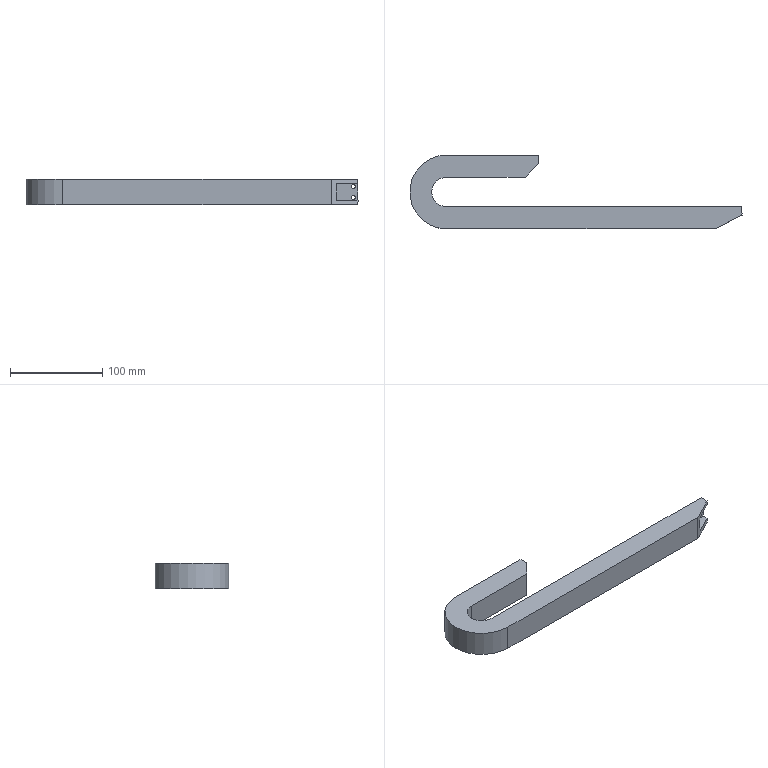Part | NX | 1 solid | 24 faces | box 360 x 80 x 28 mm | volume 171154 mm3 | plane 16 | cylinder 8 | commonest cylinder face diameters 4.5 x4 32 x1 38 x1 74 x1 80 x1
STEP:
#1=CARTESIAN_POINT('',(-232.,47.,-9.));
#2=VERTEX_POINT('',#1);
#3=CARTESIAN_POINT('',(-232.,47.,9.));
#4=VERTEX_POINT('',#3);
#5=CARTESIAN_POINT('',(-232.,47.,9.));
#6=DIRECTION('',(0.,0.,1.));
#7=VECTOR('',#6,1000.);
#8=LINE('',#5,#7);
#9=EDGE_CURVE('',#2,#4,#8,.T.);
#10=ORIENTED_EDGE('',*,*,#9,.F.);
#11=CARTESIAN_POINT('',(-320.,47.,-9.));
#12=VERTEX_POINT('',#11);
#13=CARTESIAN_POINT('',(-320.,47.,-9.));
#14=DIRECTION('',(1.,0.,0.));
#15=VECTOR('',#14,1000.);
#16=LINE('',#13,#15);
#17=EDGE_CURVE('',#12,#2,#16,.T.);
#18=ORIENTED_EDGE('',*,*,#17,.F.);
#19=CARTESIAN_POINT('',(-320.,47.,9.));
#20=VERTEX_POINT('',#19);
#21=CARTESIAN_POINT('',(-320.,47.,9.));
#22=DIRECTION('',(0.,0.,1.));
#23=VECTOR('',#22,1000.);
#24=LINE('',#21,#23);
#25=EDGE_CURVE('',#12,#20,#24,.T.);
#26=ORIENTED_EDGE('',*,*,#25,.T.);
#27=CARTESIAN_POINT('',(-320.,47.,9.));
#28=DIRECTION('',(1.,0.,0.));
#29=VECTOR('',#28,1000.);
#30=LINE('',#27,#29);
#31=EDGE_CURVE('',#20,#4,#30,.T.);
#32=ORIENTED_EDGE('',*,*,#31,.T.);
#33=EDGE_LOOP('',(#10,#18,#26,#32));
#34=FACE_BOUND('',#33,.T.);
#35=CARTESIAN_POINT('',(-320.,47.,9.));
#36=DIRECTION('',(0.,1.,0.));
#37=DIRECTION('',(0.,0.,1.));
#38=AXIS2_PLACEMENT_3D('',#35,#36,#37);
#39=PLANE('',#38);
#40=ADVANCED_FACE('',(#34),#39,.T.);
#41=CARTESIAN_POINT('',(-225.,65.,3.75));
#42=VERTEX_POINT('',#41);
#43=CARTESIAN_POINT('',(-225.,65.,6.));
#44=DIRECTION('',(0.,-1.,0.));
#45=DIRECTION('',(0.,0.,-1.));
#46=AXIS2_PLACEMENT_3D('',#43,#44,#45);
#47=CIRCLE('',#46,2.25);
#48=EDGE_CURVE('',#42,#42,#47,.T.);
#49=ORIENTED_EDGE('',*,*,#48,.F.);
#50=EDGE_LOOP('',(#49));
#51=FACE_BOUND('',#50,.T.);
#52=CARTESIAN_POINT('',(-225.,65.,-8.25));
#53=VERTEX_POINT('',#52);
#54=CARTESIAN_POINT('',(-225.,65.,-6.));
#55=DIRECTION('',(0.,-1.,0.));
#56=DIRECTION('',(0.,0.,-1.));
#57=AXIS2_PLACEMENT_3D('',#54,#55,#56);
#58=CIRCLE('',#57,2.25);
#59=EDGE_CURVE('',#53,#53,#58,.T.);
#60=ORIENTED_EDGE('',*,*,#59,.F.);
#61=EDGE_LOOP('',(#60));
#62=FACE_BOUND('',#61,.T.);
#63=CARTESIAN_POINT('',(-320.,65.,9.));
#64=VERTEX_POINT('',#63);
#65=CARTESIAN_POINT('',(-320.,65.,-9.));
#66=VERTEX_POINT('',#65);
#67=CARTESIAN_POINT('',(-320.,65.,9.));
#68=DIRECTION('',(0.,0.,-1.));
#69=VECTOR('',#68,1000.);
#70=LINE('',#67,#69);
#71=EDGE_CURVE('',#64,#66,#70,.T.);
#72=ORIENTED_EDGE('',*,*,#71,.T.);
#73=CARTESIAN_POINT('',(-220.,65.,-9.));
#74=VERTEX_POINT('',#73);
#75=CARTESIAN_POINT('',(-320.,65.,-9.));
#76=DIRECTION('',(1.,0.,0.));
#77=VECTOR('',#76,1000.);
#78=LINE('',#75,#77);
#79=EDGE_CURVE('',#66,#74,#78,.T.);
#80=ORIENTED_EDGE('',*,*,#79,.T.);
#81=CARTESIAN_POINT('',(-220.,65.,9.));
#82=VERTEX_POINT('',#81);
#83=CARTESIAN_POINT('',(-220.,65.,9.));
#84=DIRECTION('',(0.,0.,-1.));
#85=VECTOR('',#84,1000.);
#86=LINE('',#83,#85);
#87=EDGE_CURVE('',#82,#74,#86,.T.);
#88=ORIENTED_EDGE('',*,*,#87,.F.);
#89=CARTESIAN_POINT('',(-320.,65.,9.));
#90=DIRECTION('',(1.,0.,0.));
#91=VECTOR('',#90,1000.);
#92=LINE('',#89,#91);
#93=EDGE_CURVE('',#64,#82,#92,.T.);
#94=ORIENTED_EDGE('',*,*,#93,.F.);
#95=EDGE_LOOP('',(#72,#80,#88,#94));
#96=FACE_BOUND('',#95,.T.);
#97=CARTESIAN_POINT('',(-320.,65.,9.));
#98=DIRECTION('',(0.,-1.,0.));
#99=DIRECTION('',(0.,0.,-1.));
#100=AXIS2_PLACEMENT_3D('',#97,#98,#99);
#101=PLANE('',#100);
#102=ADVANCED_FACE('',(#51,#62,#96),#101,.T.);
#103=CARTESIAN_POINT('',(-225.,68.,3.75));
#104=VERTEX_POINT('',#103);
#105=CARTESIAN_POINT('',(-225.,68.,6.));
#106=DIRECTION('',(0.,-1.,0.));
#107=DIRECTION('',(0.,0.,-1.));
#108=AXIS2_PLACEMENT_3D('',#105,#106,#107);
#109=CIRCLE('',#108,2.25);
#110=EDGE_CURVE('',#104,#104,#109,.T.);
#111=ORIENTED_EDGE('',*,*,#110,.T.);
#112=EDGE_LOOP('',(#111));
#113=FACE_BOUND('',#112,.T.);
#114=CARTESIAN_POINT('',(-225.,68.,-8.25));
#115=VERTEX_POINT('',#114);
#116=CARTESIAN_POINT('',(-225.,68.,-6.));
#117=DIRECTION('',(0.,-1.,0.));
#118=DIRECTION('',(0.,0.,-1.));
#119=AXIS2_PLACEMENT_3D('',#116,#117,#118);
#120=CIRCLE('',#119,2.25);
#121=EDGE_CURVE('',#115,#115,#120,.T.);
#122=ORIENTED_EDGE('',*,*,#121,.T.);
#123=EDGE_LOOP('',(#122));
#124=FACE_BOUND('',#123,.T.);
#125=CARTESIAN_POINT('',(-320.,68.,14.));
#126=VERTEX_POINT('',#125);
#127=CARTESIAN_POINT('',(-320.,68.,-14.));
#128=VERTEX_POINT('',#127);
#129=CARTESIAN_POINT('',(-320.,68.,14.));
#130=DIRECTION('',(0.,0.,-1.));
#131=VECTOR('',#130,1000.);
#132=LINE('',#129,#131);
#133=EDGE_CURVE('',#126,#128,#132,.T.);
#134=ORIENTED_EDGE('',*,*,#133,.F.);
#135=CARTESIAN_POINT('',(-220.,68.,14.));
#136=VERTEX_POINT('',#135);
#137=CARTESIAN_POINT('',(-320.,68.,14.));
#138=DIRECTION('',(1.,0.,0.));
#139=VECTOR('',#138,1000.);
#140=LINE('',#137,#139);
#141=EDGE_CURVE('',#126,#136,#140,.T.);
#142=ORIENTED_EDGE('',*,*,#141,.T.);
#143=CARTESIAN_POINT('',(-220.,68.,-14.));
#144=VERTEX_POINT('',#143);
#145=CARTESIAN_POINT('',(-220.,68.,14.));
#146=DIRECTION('',(0.,0.,-1.));
#147=VECTOR('',#146,1000.);
#148=LINE('',#145,#147);
#149=EDGE_CURVE('',#136,#144,#148,.T.);
#150=ORIENTED_EDGE('',*,*,#149,.T.);
#151=CARTESIAN_POINT('',(-320.,68.,-14.));
#152=DIRECTION('',(1.,0.,0.));
#153=VECTOR('',#152,1000.);
#154=LINE('',#151,#153);
#155=EDGE_CURVE('',#128,#144,#154,.T.);
#156=ORIENTED_EDGE('',*,*,#155,.F.);
#157=EDGE_LOOP('',(#134,#142,#150,#156));
#158=FACE_BOUND('',#157,.T.);
#159=CARTESIAN_POINT('',(-320.,68.,14.));
#160=DIRECTION('',(0.,-1.,0.));
#161=DIRECTION('',(0.,0.,-1.));
#162=AXIS2_PLACEMENT_3D('',#159,#160,#161);
#163=PLANE('',#162);
#164=ADVANCED_FACE('',(#113,#124,#158),#163,.F.);
#165=CARTESIAN_POINT('',(-320.,44.,-14.));
#166=VERTEX_POINT('',#165);
#167=CARTESIAN_POINT('',(-235.,44.,-14.));
#168=VERTEX_POINT('',#167);
#169=CARTESIAN_POINT('',(-320.,44.,-14.));
#170=DIRECTION('',(1.,0.,0.));
#171=VECTOR('',#170,1000.);
#172=LINE('',#169,#171);
#173=EDGE_CURVE('',#166,#168,#172,.T.);
#174=ORIENTED_EDGE('',*,*,#173,.T.);
#175=CARTESIAN_POINT('',(-235.,44.,14.));
#176=VERTEX_POINT('',#175);
#177=CARTESIAN_POINT('',(-235.,44.,14.));
#178=DIRECTION('',(0.,0.,-1.));
#179=VECTOR('',#178,1000.);
#180=LINE('',#177,#179);
#181=EDGE_CURVE('',#176,#168,#180,.T.);
#182=ORIENTED_EDGE('',*,*,#181,.F.);
#183=CARTESIAN_POINT('',(-320.,44.,14.));
#184=VERTEX_POINT('',#183);
#185=CARTESIAN_POINT('',(-320.,44.,14.));
#186=DIRECTION('',(1.,0.,0.));
#187=VECTOR('',#186,1000.);
#188=LINE('',#185,#187);
#189=EDGE_CURVE('',#184,#176,#188,.T.);
#190=ORIENTED_EDGE('',*,*,#189,.F.);
#191=CARTESIAN_POINT('',(-320.,44.,14.));
#192=DIRECTION('',(0.,0.,1.));
#193=VECTOR('',#192,1000.);
#194=LINE('',#191,#193);
#195=EDGE_CURVE('',#166,#184,#194,.T.);
#196=ORIENTED_EDGE('',*,*,#195,.F.);
#197=EDGE_LOOP('',(#174,#182,#190,#196));
#198=FACE_BOUND('',#197,.T.);
#199=CARTESIAN_POINT('',(-320.,44.,14.));
#200=DIRECTION('',(0.,1.,0.));
#201=DIRECTION('',(0.,0.,1.));
#202=AXIS2_PLACEMENT_3D('',#199,#200,#201);
#203=PLANE('',#202);
#204=ADVANCED_FACE('',(#198),#203,.F.);
#205=CARTESIAN_POINT('',(-320.,9.,-9.));
#206=VERTEX_POINT('',#205);
#207=CARTESIAN_POINT('',(-320.,9.,9.));
#208=VERTEX_POINT('',#207);
#209=CARTESIAN_POINT('',(-320.,9.,9.));
#210=DIRECTION('',(0.,0.,1.));
#211=VECTOR('',#210,1000.);
#212=LINE('',#209,#211);
#213=EDGE_CURVE('',#206,#208,#212,.T.);
#214=ORIENTED_EDGE('',*,*,#213,.T.);
#215=CARTESIAN_POINT('',(-320.,28.,9.));
#216=DIRECTION('',(0.,0.,-1.));
#217=DIRECTION('',(-1.,0.,0.));
#218=AXIS2_PLACEMENT_3D('',#215,#216,#217);
#219=CIRCLE('',#218,19.);
#220=EDGE_CURVE('',#208,#20,#219,.T.);
#221=ORIENTED_EDGE('',*,*,#220,.T.);
#222=ORIENTED_EDGE('',*,*,#25,.F.);
#223=CARTESIAN_POINT('',(-320.,28.,-9.));
#224=DIRECTION('',(0.,0.,-1.));
#225=DIRECTION('',(-1.,0.,0.));
#226=AXIS2_PLACEMENT_3D('',#223,#224,#225);
#227=CIRCLE('',#226,19.);
#228=EDGE_CURVE('',#206,#12,#227,.T.);
#229=ORIENTED_EDGE('',*,*,#228,.F.);
#230=EDGE_LOOP('',(#214,#221,#222,#229));
#231=FACE_BOUND('',#230,.T.);
#232=CARTESIAN_POINT('',(-320.,28.,0.));
#233=DIRECTION('',(0.,0.,-1.));
#234=DIRECTION('',(-1.,0.,0.));
#235=AXIS2_PLACEMENT_3D('',#232,#233,#234);
#236=CYLINDRICAL_SURFACE('',#235,19.);
#237=ADVANCED_FACE('',(#231),#236,.T.);
#238=CARTESIAN_POINT('',(-320.,-9.,9.));
#239=VERTEX_POINT('',#238);
#240=CARTESIAN_POINT('',(-320.,-9.,-9.));
#241=VERTEX_POINT('',#240);
#242=CARTESIAN_POINT('',(-320.,-9.,9.));
#243=DIRECTION('',(0.,0.,-1.));
#244=VECTOR('',#243,1000.);
#245=LINE('',#242,#244);
#246=EDGE_CURVE('',#239,#241,#245,.T.);
#247=ORIENTED_EDGE('',*,*,#246,.T.);
#248=CARTESIAN_POINT('',(-320.,28.,-9.));
#249=DIRECTION('',(0.,0.,-1.));
#250=DIRECTION('',(-1.,0.,0.));
#251=AXIS2_PLACEMENT_3D('',#248,#249,#250);
#252=CIRCLE('',#251,37.);
#253=EDGE_CURVE('',#241,#66,#252,.T.);
#254=ORIENTED_EDGE('',*,*,#253,.T.);
#255=ORIENTED_EDGE('',*,*,#71,.F.);
#256=CARTESIAN_POINT('',(-320.,28.,9.));
#257=DIRECTION('',(0.,0.,-1.));
#258=DIRECTION('',(-1.,0.,0.));
#259=AXIS2_PLACEMENT_3D('',#256,#257,#258);
#260=CIRCLE('',#259,37.);
#261=EDGE_CURVE('',#239,#64,#260,.T.);
#262=ORIENTED_EDGE('',*,*,#261,.F.);
#263=EDGE_LOOP('',(#247,#254,#255,#262));
#264=FACE_BOUND('',#263,.T.);
#265=CARTESIAN_POINT('',(-320.,28.,0.));
#266=DIRECTION('',(0.,0.,-1.));
#267=DIRECTION('',(-1.,0.,0.));
#268=AXIS2_PLACEMENT_3D('',#265,#266,#267);
#269=CYLINDRICAL_SURFACE('',#268,37.);
#270=ADVANCED_FACE('',(#264),#269,.F.);
#271=CARTESIAN_POINT('',(-320.,-12.,14.));
#272=VERTEX_POINT('',#271);
#273=CARTESIAN_POINT('',(-320.,-12.,-14.));
#274=VERTEX_POINT('',#273);
#275=CARTESIAN_POINT('',(-320.,-12.,14.));
#276=DIRECTION('',(0.,0.,-1.));
#277=VECTOR('',#276,1000.);
#278=LINE('',#275,#277);
#279=EDGE_CURVE('',#272,#274,#278,.T.);
#280=ORIENTED_EDGE('',*,*,#279,.F.);
#281=CARTESIAN_POINT('',(-320.,28.,14.));
#282=DIRECTION('',(0.,0.,-1.));
#283=DIRECTION('',(-1.,0.,0.));
#284=AXIS2_PLACEMENT_3D('',#281,#282,#283);
#285=CIRCLE('',#284,40.);
#286=EDGE_CURVE('',#272,#126,#285,.T.);
#287=ORIENTED_EDGE('',*,*,#286,.T.);
#288=ORIENTED_EDGE('',*,*,#133,.T.);
#289=CARTESIAN_POINT('',(-320.,28.,-14.));
#290=DIRECTION('',(0.,0.,-1.));
#291=DIRECTION('',(-1.,0.,0.));
#292=AXIS2_PLACEMENT_3D('',#289,#290,#291);
#293=CIRCLE('',#292,40.);
#294=EDGE_CURVE('',#274,#128,#293,.T.);
#295=ORIENTED_EDGE('',*,*,#294,.F.);
#296=EDGE_LOOP('',(#280,#287,#288,#295));
#297=FACE_BOUND('',#296,.T.);
#298=CARTESIAN_POINT('',(-320.,28.,0.));
#299=DIRECTION('',(0.,0.,-1.));
#300=DIRECTION('',(-1.,0.,0.));
#301=AXIS2_PLACEMENT_3D('',#298,#299,#300);
#302=CYLINDRICAL_SURFACE('',#301,40.);
#303=ADVANCED_FACE('',(#297),#302,.T.);
#304=CARTESIAN_POINT('',(-320.,12.,-14.));
#305=VERTEX_POINT('',#304);
#306=CARTESIAN_POINT('',(-320.,12.,14.));
#307=VERTEX_POINT('',#306);
#308=CARTESIAN_POINT('',(-320.,12.,14.));
#309=DIRECTION('',(0.,0.,1.));
#310=VECTOR('',#309,1000.);
#311=LINE('',#308,#310);
#312=EDGE_CURVE('',#305,#307,#311,.T.);
#313=ORIENTED_EDGE('',*,*,#312,.F.);
#314=CARTESIAN_POINT('',(-320.,28.,-14.));
#315=DIRECTION('',(0.,0.,-1.));
#316=DIRECTION('',(-1.,0.,0.));
#317=AXIS2_PLACEMENT_3D('',#314,#315,#316);
#318=CIRCLE('',#317,16.);
#319=EDGE_CURVE('',#305,#166,#318,.T.);
#320=ORIENTED_EDGE('',*,*,#319,.T.);
#321=ORIENTED_EDGE('',*,*,#195,.T.);
#322=CARTESIAN_POINT('',(-320.,28.,14.));
#323=DIRECTION('',(0.,0.,-1.));
#324=DIRECTION('',(-1.,0.,0.));
#325=AXIS2_PLACEMENT_3D('',#322,#323,#324);
#326=CIRCLE('',#325,16.);
#327=EDGE_CURVE('',#307,#184,#326,.T.);
#328=ORIENTED_EDGE('',*,*,#327,.F.);
#329=EDGE_LOOP('',(#313,#320,#321,#328));
#330=FACE_BOUND('',#329,.T.);
#331=CARTESIAN_POINT('',(-320.,28.,0.));
#332=DIRECTION('',(0.,0.,-1.));
#333=DIRECTION('',(-1.,0.,0.));
#334=AXIS2_PLACEMENT_3D('',#331,#332,#333);
#335=CYLINDRICAL_SURFACE('',#334,16.);
#336=ADVANCED_FACE('',(#330),#335,.F.);
#337=CARTESIAN_POINT('',(-23.124,-9.,-9.));
#338=VERTEX_POINT('',#337);
#339=CARTESIAN_POINT('',(-320.,-9.,-9.));
#340=DIRECTION('',(1.,0.,0.));
#341=VECTOR('',#340,1000.);
#342=LINE('',#339,#341);
#343=EDGE_CURVE('',#241,#338,#342,.T.);
#344=ORIENTED_EDGE('',*,*,#343,.T.);
#345=CARTESIAN_POINT('',(0.,3.,-9.));
#346=VERTEX_POINT('',#345);
#347=CARTESIAN_POINT('',(-257.012,-130.376,-9.));
#348=DIRECTION('',(0.8876,0.4606,0.));
#349=VECTOR('',#348,1000.);
#350=LINE('',#347,#349);
#351=EDGE_CURVE('',#338,#346,#350,.T.);
#352=ORIENTED_EDGE('',*,*,#351,.T.);
#353=CARTESIAN_POINT('',(0.,9.,-9.));
#354=VERTEX_POINT('',#353);
#355=CARTESIAN_POINT('',(0.,-9.,-9.));
#356=DIRECTION('',(0.,1.,0.));
#357=VECTOR('',#356,1000.);
#358=LINE('',#355,#357);
#359=EDGE_CURVE('',#346,#354,#358,.T.);
#360=ORIENTED_EDGE('',*,*,#359,.T.);
#361=CARTESIAN_POINT('',(-320.,9.,-9.));
#362=DIRECTION('',(1.,0.,0.));
#363=VECTOR('',#362,1000.);
#364=LINE('',#361,#363);
#365=EDGE_CURVE('',#206,#354,#364,.T.);
#366=ORIENTED_EDGE('',*,*,#365,.F.);
#367=ORIENTED_EDGE('',*,*,#228,.T.);
#368=ORIENTED_EDGE('',*,*,#17,.T.);
#369=CARTESIAN_POINT('',(-220.,59.,-9.));
#370=VERTEX_POINT('',#369);
#371=CARTESIAN_POINT('',(-304.,-25.,-9.));
#372=DIRECTION('',(0.7071,0.7071,0.));
#373=VECTOR('',#372,1000.);
#374=LINE('',#371,#373);
#375=EDGE_CURVE('',#2,#370,#374,.T.);
#376=ORIENTED_EDGE('',*,*,#375,.T.);
#377=CARTESIAN_POINT('',(-220.,65.,-9.));
#378=DIRECTION('',(0.,-1.,0.));
#379=VECTOR('',#378,1000.);
#380=LINE('',#377,#379);
#381=EDGE_CURVE('',#74,#370,#380,.T.);
#382=ORIENTED_EDGE('',*,*,#381,.F.);
#383=ORIENTED_EDGE('',*,*,#79,.F.);
#384=ORIENTED_EDGE('',*,*,#253,.F.);
#385=EDGE_LOOP('',(#344,#352,#360,#366,#367,#368,#376,#382,#383,#384));
#386=FACE_BOUND('',#385,.T.);
#387=CARTESIAN_POINT('',(-320.,-9.,-9.));
#388=DIRECTION('',(0.,0.,-1.));
#389=DIRECTION('',(-1.,0.,0.));
#390=AXIS2_PLACEMENT_3D('',#387,#388,#389);
#391=PLANE('',#390);
#392=ADVANCED_FACE('',(#386),#391,.F.);
#393=CARTESIAN_POINT('',(-7.25,9.,6.));
#394=VERTEX_POINT('',#393);
#395=CARTESIAN_POINT('',(-5.,9.,6.));
#396=DIRECTION('',(0.,1.,0.));
#397=DIRECTION('',(-1.,0.,0.));
#398=AXIS2_PLACEMENT_3D('',#395,#396,#397);
#399=CIRCLE('',#398,2.25);
#400=EDGE_CURVE('',#394,#394,#399,.T.);
#401=ORIENTED_EDGE('',*,*,#400,.T.);
#402=EDGE_LOOP('',(#401));
#403=FACE_BOUND('',#402,.T.);
#404=CARTESIAN_POINT('',(-7.25,9.,-6.));
#405=VERTEX_POINT('',#404);
#406=CARTESIAN_POINT('',(-5.,9.,-6.));
#407=DIRECTION('',(0.,1.,0.));
#408=DIRECTION('',(-1.,0.,0.));
#409=AXIS2_PLACEMENT_3D('',#406,#407,#408);
#410=CIRCLE('',#409,2.25);
#411=EDGE_CURVE('',#405,#405,#410,.T.);
#412=ORIENTED_EDGE('',*,*,#411,.T.);
#413=EDGE_LOOP('',(#412));
#414=FACE_BOUND('',#413,.T.);
#415=CARTESIAN_POINT('',(0.,9.,9.));
#416=VERTEX_POINT('',#415);
#417=CARTESIAN_POINT('',(0.,9.,9.));
#418=DIRECTION('',(0.,0.,1.));
#419=VECTOR('',#418,1000.);
#420=LINE('',#417,#419);
#421=EDGE_CURVE('',#354,#416,#420,.T.);
#422=ORIENTED_EDGE('',*,*,#421,.T.);
#423=CARTESIAN_POINT('',(-320.,9.,9.));
#424=DIRECTION('',(1.,0.,0.));
#425=VECTOR('',#424,1000.);
#426=LINE('',#423,#425);
#427=EDGE_CURVE('',#208,#416,#426,.T.);
#428=ORIENTED_EDGE('',*,*,#427,.F.);
#429=ORIENTED_EDGE('',*,*,#213,.F.);
#430=ORIENTED_EDGE('',*,*,#365,.T.);
#431=EDGE_LOOP('',(#422,#428,#429,#430));
#432=FACE_BOUND('',#431,.T.);
#433=CARTESIAN_POINT('',(-320.,9.,9.));
#434=DIRECTION('',(0.,1.,0.));
#435=DIRECTION('',(-1.,0.,0.));
#436=AXIS2_PLACEMENT_3D('',#433,#434,#435);
#437=PLANE('',#436);
#438=ADVANCED_FACE('',(#403,#414,#432),#437,.F.);
#439=CARTESIAN_POINT('',(0.,3.,9.));
#440=VERTEX_POINT('',#439);
#441=CARTESIAN_POINT('',(0.,-9.,9.));
#442=DIRECTION('',(0.,-1.,0.));
#443=VECTOR('',#442,1000.);
#444=LINE('',#441,#443);
#445=EDGE_CURVE('',#416,#440,#444,.T.);
#446=ORIENTED_EDGE('',*,*,#445,.T.);
#447=CARTESIAN_POINT('',(-23.124,-9.,9.));
#448=VERTEX_POINT('',#447);
#449=CARTESIAN_POINT('',(-257.012,-130.376,9.));
#450=DIRECTION('',(-0.8876,-0.4606,0.));
#451=VECTOR('',#450,1000.);
#452=LINE('',#449,#451);
#453=EDGE_CURVE('',#440,#448,#452,.T.);
#454=ORIENTED_EDGE('',*,*,#453,.T.);
#455=CARTESIAN_POINT('',(-320.,-9.,9.));
#456=DIRECTION('',(1.,0.,0.));
#457=VECTOR('',#456,1000.);
#458=LINE('',#455,#457);
#459=EDGE_CURVE('',#239,#448,#458,.T.);
#460=ORIENTED_EDGE('',*,*,#459,.F.);
#461=ORIENTED_EDGE('',*,*,#261,.T.);
#462=ORIENTED_EDGE('',*,*,#93,.T.);
#463=CARTESIAN_POINT('',(-220.,59.,9.));
#464=VERTEX_POINT('',#463);
#465=CARTESIAN_POINT('',(-220.,65.,9.));
#466=DIRECTION('',(0.,1.,0.));
#467=VECTOR('',#466,1000.);
#468=LINE('',#465,#467);
#469=EDGE_CURVE('',#464,#82,#468,.T.);
#470=ORIENTED_EDGE('',*,*,#469,.F.);
#471=CARTESIAN_POINT('',(-304.,-25.,9.));
#472=DIRECTION('',(-0.7071,-0.7071,0.));
#473=VECTOR('',#472,1000.);
#474=LINE('',#471,#473);
#475=EDGE_CURVE('',#464,#4,#474,.T.);
#476=ORIENTED_EDGE('',*,*,#475,.T.);
#477=ORIENTED_EDGE('',*,*,#31,.F.);
#478=ORIENTED_EDGE('',*,*,#220,.F.);
#479=ORIENTED_EDGE('',*,*,#427,.T.);
#480=EDGE_LOOP('',(#446,#454,#460,#461,#462,#470,#476,#477,#478,#479));
#481=FACE_BOUND('',#480,.T.);
#482=CARTESIAN_POINT('',(-320.,-9.,9.));
#483=DIRECTION('',(0.,0.,1.));
#484=DIRECTION('',(1.,0.,0.));
#485=AXIS2_PLACEMENT_3D('',#482,#483,#484);
#486=PLANE('',#485);
#487=ADVANCED_FACE('',(#481),#486,.F.);
#488=CARTESIAN_POINT('',(0.,3.,-14.));
#489=VERTEX_POINT('',#488);
#490=CARTESIAN_POINT('',(-28.905,-12.,-14.));
#491=VERTEX_POINT('',#490);
#492=CARTESIAN_POINT('',(0.,3.,-14.));
#493=DIRECTION('',(-0.8876,-0.4606,0.));
#494=VECTOR('',#493,1000.);
#495=LINE('',#492,#494);
#496=EDGE_CURVE('',#489,#491,#495,.T.);
#497=ORIENTED_EDGE('',*,*,#496,.T.);
#498=CARTESIAN_POINT('',(-320.,-12.,-14.));
#499=DIRECTION('',(1.,0.,0.));
#500=VECTOR('',#499,1000.);
#501=LINE('',#498,#500);
#502=EDGE_CURVE('',#274,#491,#501,.T.);
#503=ORIENTED_EDGE('',*,*,#502,.F.);
#504=ORIENTED_EDGE('',*,*,#294,.T.);
#505=ORIENTED_EDGE('',*,*,#155,.T.);
#506=CARTESIAN_POINT('',(-220.,59.,-14.));
#507=VERTEX_POINT('',#506);
#508=CARTESIAN_POINT('',(-220.,68.,-14.));
#509=DIRECTION('',(0.,-1.,0.));
#510=VECTOR('',#509,1000.);
#511=LINE('',#508,#510);
#512=EDGE_CURVE('',#144,#507,#511,.T.);
#513=ORIENTED_EDGE('',*,*,#512,.T.);
#514=CARTESIAN_POINT('',(-220.,59.,-14.));
#515=DIRECTION('',(0.7071,0.7071,0.));
#516=VECTOR('',#515,1000.);
#517=LINE('',#514,#516);
#518=EDGE_CURVE('',#168,#507,#517,.T.);
#519=ORIENTED_EDGE('',*,*,#518,.F.);
#520=ORIENTED_EDGE('',*,*,#173,.F.);
#521=ORIENTED_EDGE('',*,*,#319,.F.);
#522=CARTESIAN_POINT('',(0.,12.,-14.));
#523=VERTEX_POINT('',#522);
#524=CARTESIAN_POINT('',(-320.,12.,-14.));
#525=DIRECTION('',(1.,0.,0.));
#526=VECTOR('',#525,1000.);
#527=LINE('',#524,#526);
#528=EDGE_CURVE('',#305,#523,#527,.T.);
#529=ORIENTED_EDGE('',*,*,#528,.T.);
#530=CARTESIAN_POINT('',(0.,-12.,-14.));
#531=DIRECTION('',(0.,1.,0.));
#532=VECTOR('',#531,1000.);
#533=LINE('',#530,#532);
#534=EDGE_CURVE('',#489,#523,#533,.T.);
#535=ORIENTED_EDGE('',*,*,#534,.F.);
#536=EDGE_LOOP('',(#497,#503,#504,#505,#513,#519,#520,#521,#529,#535));
#537=FACE_BOUND('',#536,.T.);
#538=CARTESIAN_POINT('',(-320.,-12.,-14.));
#539=DIRECTION('',(0.,0.,-1.));
#540=DIRECTION('',(-1.,0.,0.));
#541=AXIS2_PLACEMENT_3D('',#538,#539,#540);
#542=PLANE('',#541);
#543=ADVANCED_FACE('',(#537),#542,.T.);
#544=CARTESIAN_POINT('',(-28.905,-12.,14.));
#545=VERTEX_POINT('',#544);
#546=CARTESIAN_POINT('',(-28.905,-12.,-14.));
#547=DIRECTION('',(0.,0.,1.));
#548=VECTOR('',#547,1000.);
#549=LINE('',#546,#548);
#550=EDGE_CURVE('',#491,#545,#549,.T.);
#551=ORIENTED_EDGE('',*,*,#550,.T.);
#552=CARTESIAN_POINT('',(-320.,-12.,14.));
#553=DIRECTION('',(1.,0.,0.));
#554=VECTOR('',#553,1000.);
#555=LINE('',#552,#554);
#556=EDGE_CURVE('',#272,#545,#555,.T.);
#557=ORIENTED_EDGE('',*,*,#556,.F.);
#558=ORIENTED_EDGE('',*,*,#279,.T.);
#559=ORIENTED_EDGE('',*,*,#502,.T.);
#560=EDGE_LOOP('',(#551,#557,#558,#559));
#561=FACE_BOUND('',#560,.T.);
#562=CARTESIAN_POINT('',(-320.,-12.,14.));
#563=DIRECTION('',(0.,-1.,0.));
#564=DIRECTION('',(1.,0.,0.));
#565=AXIS2_PLACEMENT_3D('',#562,#563,#564);
#566=PLANE('',#565);
#567=ADVANCED_FACE('',(#561),#566,.T.);
#568=CARTESIAN_POINT('',(0.,3.,14.));
#569=VERTEX_POINT('',#568);
#570=CARTESIAN_POINT('',(0.,3.,14.));
#571=DIRECTION('',(-0.8876,-0.4606,0.));
#572=VECTOR('',#571,1000.);
#573=LINE('',#570,#572);
#574=EDGE_CURVE('',#569,#545,#573,.T.);
#575=ORIENTED_EDGE('',*,*,#574,.F.);
#576=CARTESIAN_POINT('',(0.,12.,14.));
#577=VERTEX_POINT('',#576);
#578=CARTESIAN_POINT('',(0.,-12.,14.));
#579=DIRECTION('',(0.,-1.,0.));
#580=VECTOR('',#579,1000.);
#581=LINE('',#578,#580);
#582=EDGE_CURVE('',#577,#569,#581,.T.);
#583=ORIENTED_EDGE('',*,*,#582,.F.);
#584=CARTESIAN_POINT('',(-320.,12.,14.));
#585=DIRECTION('',(1.,0.,0.));
#586=VECTOR('',#585,1000.);
#587=LINE('',#584,#586);
#588=EDGE_CURVE('',#307,#577,#587,.T.);
#589=ORIENTED_EDGE('',*,*,#588,.F.);
#590=ORIENTED_EDGE('',*,*,#327,.T.);
#591=ORIENTED_EDGE('',*,*,#189,.T.);
#592=CARTESIAN_POINT('',(-220.,59.,14.));
#593=VERTEX_POINT('',#592);
#594=CARTESIAN_POINT('',(-220.,59.,14.));
#595=DIRECTION('',(0.7071,0.7071,0.));
#596=VECTOR('',#595,1000.);
#597=LINE('',#594,#596);
#598=EDGE_CURVE('',#176,#593,#597,.T.);
#599=ORIENTED_EDGE('',*,*,#598,.T.);
#600=CARTESIAN_POINT('',(-220.,68.,14.));
#601=DIRECTION('',(0.,1.,0.));
#602=VECTOR('',#601,1000.);
#603=LINE('',#600,#602);
#604=EDGE_CURVE('',#593,#136,#603,.T.);
#605=ORIENTED_EDGE('',*,*,#604,.T.);
#606=ORIENTED_EDGE('',*,*,#141,.F.);
#607=ORIENTED_EDGE('',*,*,#286,.F.);
#608=ORIENTED_EDGE('',*,*,#556,.T.);
#609=EDGE_LOOP('',(#575,#583,#589,#590,#591,#599,#605,#606,#607,#608));
#610=FACE_BOUND('',#609,.T.);
#611=CARTESIAN_POINT('',(-320.,-12.,14.));
#612=DIRECTION('',(0.,0.,1.));
#613=DIRECTION('',(1.,0.,0.));
#614=AXIS2_PLACEMENT_3D('',#611,#612,#613);
#615=PLANE('',#614);
#616=ADVANCED_FACE('',(#610),#615,.T.);
#617=CARTESIAN_POINT('',(-7.25,12.,6.));
#618=VERTEX_POINT('',#617);
#619=CARTESIAN_POINT('',(-5.,12.,6.));
#620=DIRECTION('',(0.,1.,0.));
#621=DIRECTION('',(-1.,0.,0.));
#622=AXIS2_PLACEMENT_3D('',#619,#620,#621);
#623=CIRCLE('',#622,2.25);
#624=EDGE_CURVE('',#618,#618,#623,.T.);
#625=ORIENTED_EDGE('',*,*,#624,.F.);
#626=EDGE_LOOP('',(#625));
#627=FACE_BOUND('',#626,.T.);
#628=CARTESIAN_POINT('',(-7.25,12.,-6.));
#629=VERTEX_POINT('',#628);
#630=CARTESIAN_POINT('',(-5.,12.,-6.));
#631=DIRECTION('',(0.,1.,0.));
#632=DIRECTION('',(-1.,0.,0.));
#633=AXIS2_PLACEMENT_3D('',#630,#631,#632);
#634=CIRCLE('',#633,2.25);
#635=EDGE_CURVE('',#629,#629,#634,.T.);
#636=ORIENTED_EDGE('',*,*,#635,.F.);
#637=EDGE_LOOP('',(#636));
#638=FACE_BOUND('',#637,.T.);
#639=CARTESIAN_POINT('',(0.,12.,14.));
#640=DIRECTION('',(0.,0.,1.));
#641=VECTOR('',#640,1000.);
#642=LINE('',#639,#641);
#643=EDGE_CURVE('',#523,#577,#642,.T.);
#644=ORIENTED_EDGE('',*,*,#643,.F.);
#645=ORIENTED_EDGE('',*,*,#528,.F.);
#646=ORIENTED_EDGE('',*,*,#312,.T.);
#647=ORIENTED_EDGE('',*,*,#588,.T.);
#648=EDGE_LOOP('',(#644,#645,#646,#647));
#649=FACE_BOUND('',#648,.T.);
#650=CARTESIAN_POINT('',(-320.,12.,14.));
#651=DIRECTION('',(0.,1.,0.));
#652=DIRECTION('',(-1.,0.,0.));
#653=AXIS2_PLACEMENT_3D('',#650,#651,#652);
#654=PLANE('',#653);
#655=ADVANCED_FACE('',(#627,#638,#649),#654,.T.);
#656=ORIENTED_EDGE('',*,*,#459,.T.);
#657=CARTESIAN_POINT('',(-23.124,-9.,9.));
#658=DIRECTION('',(0.,0.,-1.));
#659=VECTOR('',#658,1000.);
#660=LINE('',#657,#659);
#661=EDGE_CURVE('',#448,#338,#660,.T.);
#662=ORIENTED_EDGE('',*,*,#661,.T.);
#663=ORIENTED_EDGE('',*,*,#343,.F.);
#664=ORIENTED_EDGE('',*,*,#246,.F.);
#665=EDGE_LOOP('',(#656,#662,#663,#664));
#666=FACE_BOUND('',#665,.T.);
#667=CARTESIAN_POINT('',(-320.,-9.,9.));
#668=DIRECTION('',(0.,-1.,0.));
#669=DIRECTION('',(1.,0.,0.));
#670=AXIS2_PLACEMENT_3D('',#667,#668,#669);
#671=PLANE('',#670);
#672=ADVANCED_FACE('',(#666),#671,.F.);
#673=CARTESIAN_POINT('',(-220.,59.,0.));
#674=DIRECTION('',(0.,0.,1.));
#675=VECTOR('',#674,1000.);
#676=LINE('',#673,#675);
#677=EDGE_CURVE('',#507,#370,#676,.T.);
#678=ORIENTED_EDGE('',*,*,#677,.F.);
#679=ORIENTED_EDGE('',*,*,#512,.F.);
#680=ORIENTED_EDGE('',*,*,#149,.F.);
#681=ORIENTED_EDGE('',*,*,#604,.F.);
#682=CARTESIAN_POINT('',(-220.,59.,14.));
#683=DIRECTION('',(0.,0.,-1.));
#684=VECTOR('',#683,1000.);
#685=LINE('',#682,#684);
#686=EDGE_CURVE('',#464,#593,#685,.F.);
#687=ORIENTED_EDGE('',*,*,#686,.F.);
#688=ORIENTED_EDGE('',*,*,#469,.T.);
#689=ORIENTED_EDGE('',*,*,#87,.T.);
#690=ORIENTED_EDGE('',*,*,#381,.T.);
#691=EDGE_LOOP('',(#678,#679,#680,#681,#687,#688,#689,#690));
#692=FACE_BOUND('',#691,.T.);
#693=CARTESIAN_POINT('',(-220.,56.,0.));
#694=DIRECTION('',(1.,0.,0.));
#695=DIRECTION('',(0.,0.,1.));
#696=AXIS2_PLACEMENT_3D('',#693,#694,#695);
#697=PLANE('',#696);
#698=ADVANCED_FACE('',(#692),#697,.T.);
#699=ORIENTED_EDGE('',*,*,#582,.T.);
#700=CARTESIAN_POINT('',(0.,3.,0.));
#701=DIRECTION('',(0.,0.,-1.));
#702=VECTOR('',#701,1000.);
#703=LINE('',#700,#702);
#704=EDGE_CURVE('',#440,#569,#703,.F.);
#705=ORIENTED_EDGE('',*,*,#704,.F.);
#706=ORIENTED_EDGE('',*,*,#445,.F.);
#707=ORIENTED_EDGE('',*,*,#421,.F.);
#708=ORIENTED_EDGE('',*,*,#359,.F.);
#709=CARTESIAN_POINT('',(0.,3.,-14.));
#710=DIRECTION('',(0.,0.,1.));
#711=VECTOR('',#710,1000.);
#712=LINE('',#709,#711);
#713=EDGE_CURVE('',#489,#346,#712,.T.);
#714=ORIENTED_EDGE('',*,*,#713,.F.);
#715=ORIENTED_EDGE('',*,*,#534,.T.);
#716=ORIENTED_EDGE('',*,*,#643,.T.);
#717=EDGE_LOOP('',(#699,#705,#706,#707,#708,#714,#715,#716));
#718=FACE_BOUND('',#717,.T.);
#719=CARTESIAN_POINT('',(0.,0.,0.));
#720=DIRECTION('',(-1.,0.,0.));
#721=DIRECTION('',(0.,0.,1.));
#722=AXIS2_PLACEMENT_3D('',#719,#720,#721);
#723=PLANE('',#722);
#724=ADVANCED_FACE('',(#718),#723,.F.);
#725=ORIENTED_EDGE('',*,*,#9,.T.);
#726=ORIENTED_EDGE('',*,*,#475,.F.);
#727=ORIENTED_EDGE('',*,*,#686,.T.);
#728=ORIENTED_EDGE('',*,*,#598,.F.);
#729=ORIENTED_EDGE('',*,*,#181,.T.);
#730=ORIENTED_EDGE('',*,*,#518,.T.);
#731=ORIENTED_EDGE('',*,*,#677,.T.);
#732=ORIENTED_EDGE('',*,*,#375,.F.);
#733=EDGE_LOOP('',(#725,#726,#727,#728,#729,#730,#731,#732));
#734=FACE_BOUND('',#733,.T.);
#735=CARTESIAN_POINT('',(-220.,59.,14.));
#736=DIRECTION('',(-0.7071,0.7071,0.));
#737=DIRECTION('',(-0.7071,-0.7071,0.));
#738=AXIS2_PLACEMENT_3D('',#735,#736,#737);
#739=PLANE('',#738);
#740=ADVANCED_FACE('',(#734),#739,.F.);
#741=ORIENTED_EDGE('',*,*,#661,.F.);
#742=ORIENTED_EDGE('',*,*,#453,.F.);
#743=ORIENTED_EDGE('',*,*,#704,.T.);
#744=ORIENTED_EDGE('',*,*,#574,.T.);
#745=ORIENTED_EDGE('',*,*,#550,.F.);
#746=ORIENTED_EDGE('',*,*,#496,.F.);
#747=ORIENTED_EDGE('',*,*,#713,.T.);
#748=ORIENTED_EDGE('',*,*,#351,.F.);
#749=EDGE_LOOP('',(#741,#742,#743,#744,#745,#746,#747,#748));
#750=FACE_BOUND('',#749,.T.);
#751=CARTESIAN_POINT('',(0.,3.,-14.));
#752=DIRECTION('',(-0.4606,0.8876,0.));
#753=DIRECTION('',(-0.8876,-0.4606,0.));
#754=AXIS2_PLACEMENT_3D('',#751,#752,#753);
#755=PLANE('',#754);
#756=ADVANCED_FACE('',(#750),#755,.F.);
#757=ORIENTED_EDGE('',*,*,#635,.T.);
#758=EDGE_LOOP('',(#757));
#759=FACE_BOUND('',#758,.T.);
#760=ORIENTED_EDGE('',*,*,#411,.F.);
#761=EDGE_LOOP('',(#760));
#762=FACE_BOUND('',#761,.T.);
#763=CARTESIAN_POINT('',(-5.,-9.,-6.));
#764=DIRECTION('',(0.,-1.,0.));
#765=DIRECTION('',(0.,0.,-1.));
#766=AXIS2_PLACEMENT_3D('',#763,#764,#765);
#767=CYLINDRICAL_SURFACE('',#766,2.25);
#768=ADVANCED_FACE('',(#759,#762),#767,.F.);
#769=ORIENTED_EDGE('',*,*,#624,.T.);
#770=EDGE_LOOP('',(#769));
#771=FACE_BOUND('',#770,.T.);
#772=ORIENTED_EDGE('',*,*,#400,.F.);
#773=EDGE_LOOP('',(#772));
#774=FACE_BOUND('',#773,.T.);
#775=CARTESIAN_POINT('',(-5.,-9.,6.));
#776=DIRECTION('',(0.,-1.,0.));
#777=DIRECTION('',(0.,0.,-1.));
#778=AXIS2_PLACEMENT_3D('',#775,#776,#777);
#779=CYLINDRICAL_SURFACE('',#778,2.25);
#780=ADVANCED_FACE('',(#771,#774),#779,.F.);
#781=ORIENTED_EDGE('',*,*,#121,.F.);
#782=EDGE_LOOP('',(#781));
#783=FACE_BOUND('',#782,.T.);
#784=ORIENTED_EDGE('',*,*,#59,.T.);
#785=EDGE_LOOP('',(#784));
#786=FACE_BOUND('',#785,.T.);
#787=CARTESIAN_POINT('',(-225.,65.,-6.));
#788=DIRECTION('',(0.,-1.,0.));
#789=DIRECTION('',(0.,0.,-1.));
#790=AXIS2_PLACEMENT_3D('',#787,#788,#789);
#791=CYLINDRICAL_SURFACE('',#790,2.25);
#792=ADVANCED_FACE('',(#783,#786),#791,.F.);
#793=ORIENTED_EDGE('',*,*,#110,.F.);
#794=EDGE_LOOP('',(#793));
#795=FACE_BOUND('',#794,.T.);
#796=ORIENTED_EDGE('',*,*,#48,.T.);
#797=EDGE_LOOP('',(#796));
#798=FACE_BOUND('',#797,.T.);
#799=CARTESIAN_POINT('',(-225.,65.,6.));
#800=DIRECTION('',(0.,-1.,0.));
#801=DIRECTION('',(0.,0.,-1.));
#802=AXIS2_PLACEMENT_3D('',#799,#800,#801);
#803=CYLINDRICAL_SURFACE('',#802,2.25);
#804=ADVANCED_FACE('',(#795,#798),#803,.F.);
#805=CLOSED_SHELL('',(#40,#102,#164,#204,#237,#270,#303,#336,#392,#438,#487,#543,#567,#616,#655,#672,#698,#724,#740,#756,#768,#780,#792,#804));
#806=MANIFOLD_SOLID_BREP('',#805);
#807=(LENGTH_UNIT()NAMED_UNIT(*)SI_UNIT(.MILLI.,.METRE.));
#808=UNCERTAINTY_MEASURE_WITH_UNIT(LENGTH_MEASURE(0.00001),#807,'','');
#809=(NAMED_UNIT(*)PLANE_ANGLE_UNIT()SI_UNIT($,.RADIAN.));
#810=(NAMED_UNIT(*)SI_UNIT($,.STERADIAN.)SOLID_ANGLE_UNIT());
#811=(GEOMETRIC_REPRESENTATION_CONTEXT(3)GLOBAL_UNCERTAINTY_ASSIGNED_CONTEXT((#808))GLOBAL_UNIT_ASSIGNED_CONTEXT((#807,#809,#810))REPRESENTATION_CONTEXT('',''));
#812=ADVANCED_BREP_SHAPE_REPRESENTATION('',(#806),#811);